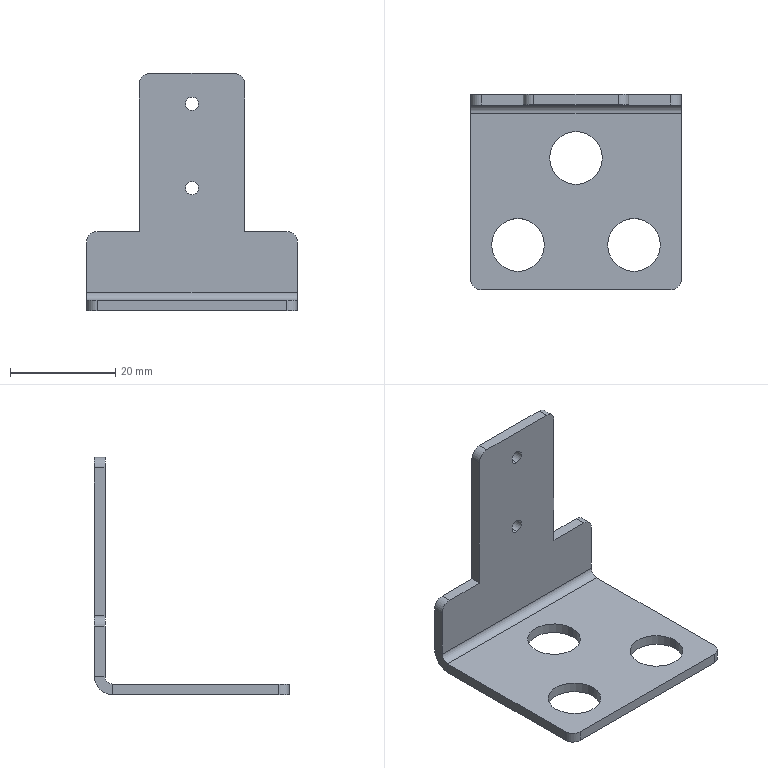Part | STEP file | PN_0038 Sensor BKT_Default | 1 solid | 34 faces | box 40 x 37 x 45 mm | volume 4613 mm3 | cylinder 18 | plane 16 | commonest cylinder face diameters 4 x6 10 x6 2.5 x4 3 x1 7 x1